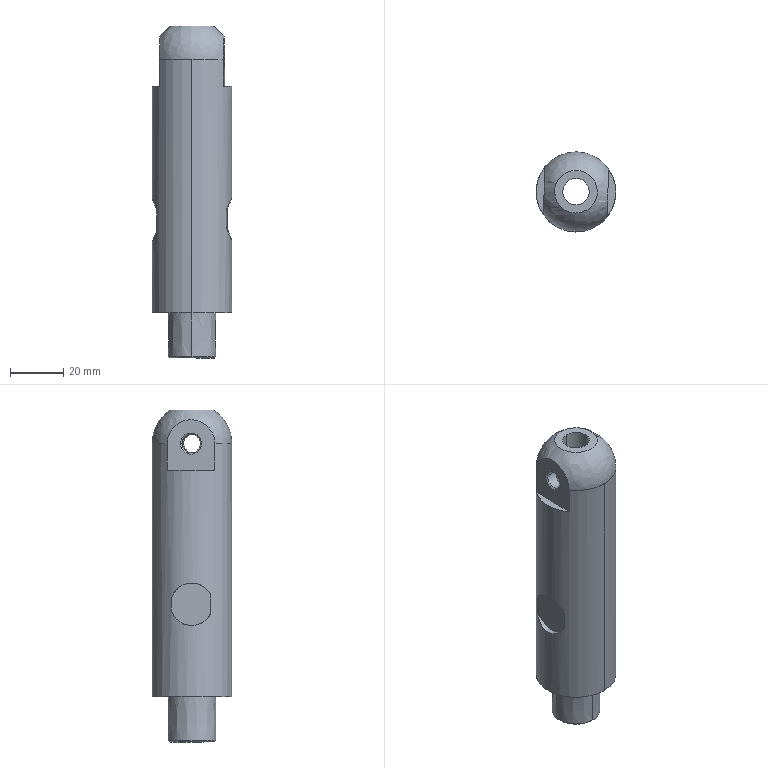Part | SolidWorks | features BaseBody 1 | 1 solid | 35 faces | box 30 x 30 x 125.047 mm | volume 52499 mm3 | cylinder 14 | cone 10 | plane 8 | spline 3 | commonest cylinder face diameters 16 x6 7 x4 10 x2 30 x2